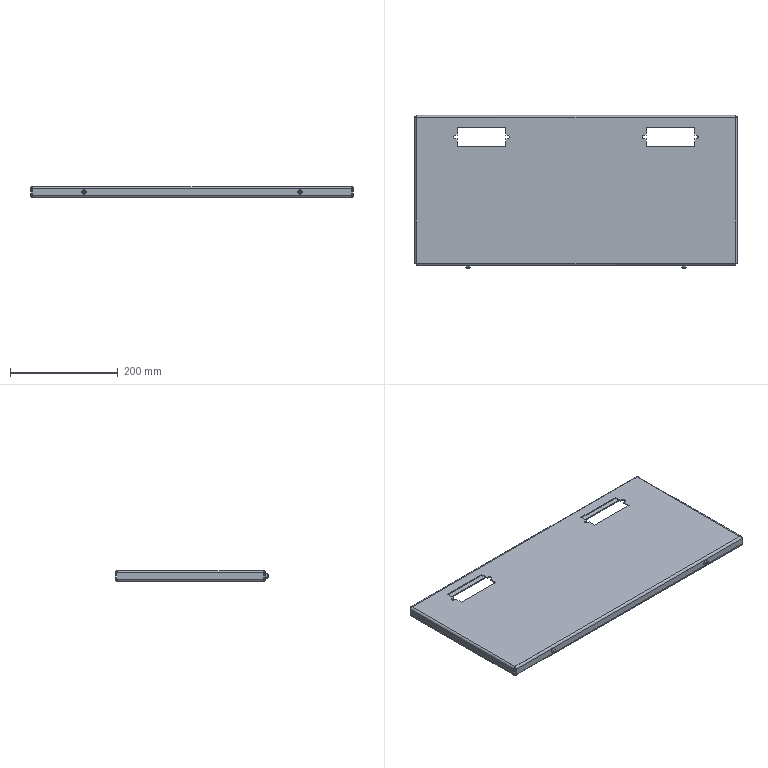Part | NX | features BREP 1 | 1 solid | 106 faces | box 598 x 284 x 20 mm | volume 416605 mm3 | plane 60 | cylinder 26 | spline 16 | cone 4 | commonest cylinder face diameters 8 x12 4 x8 7 x6